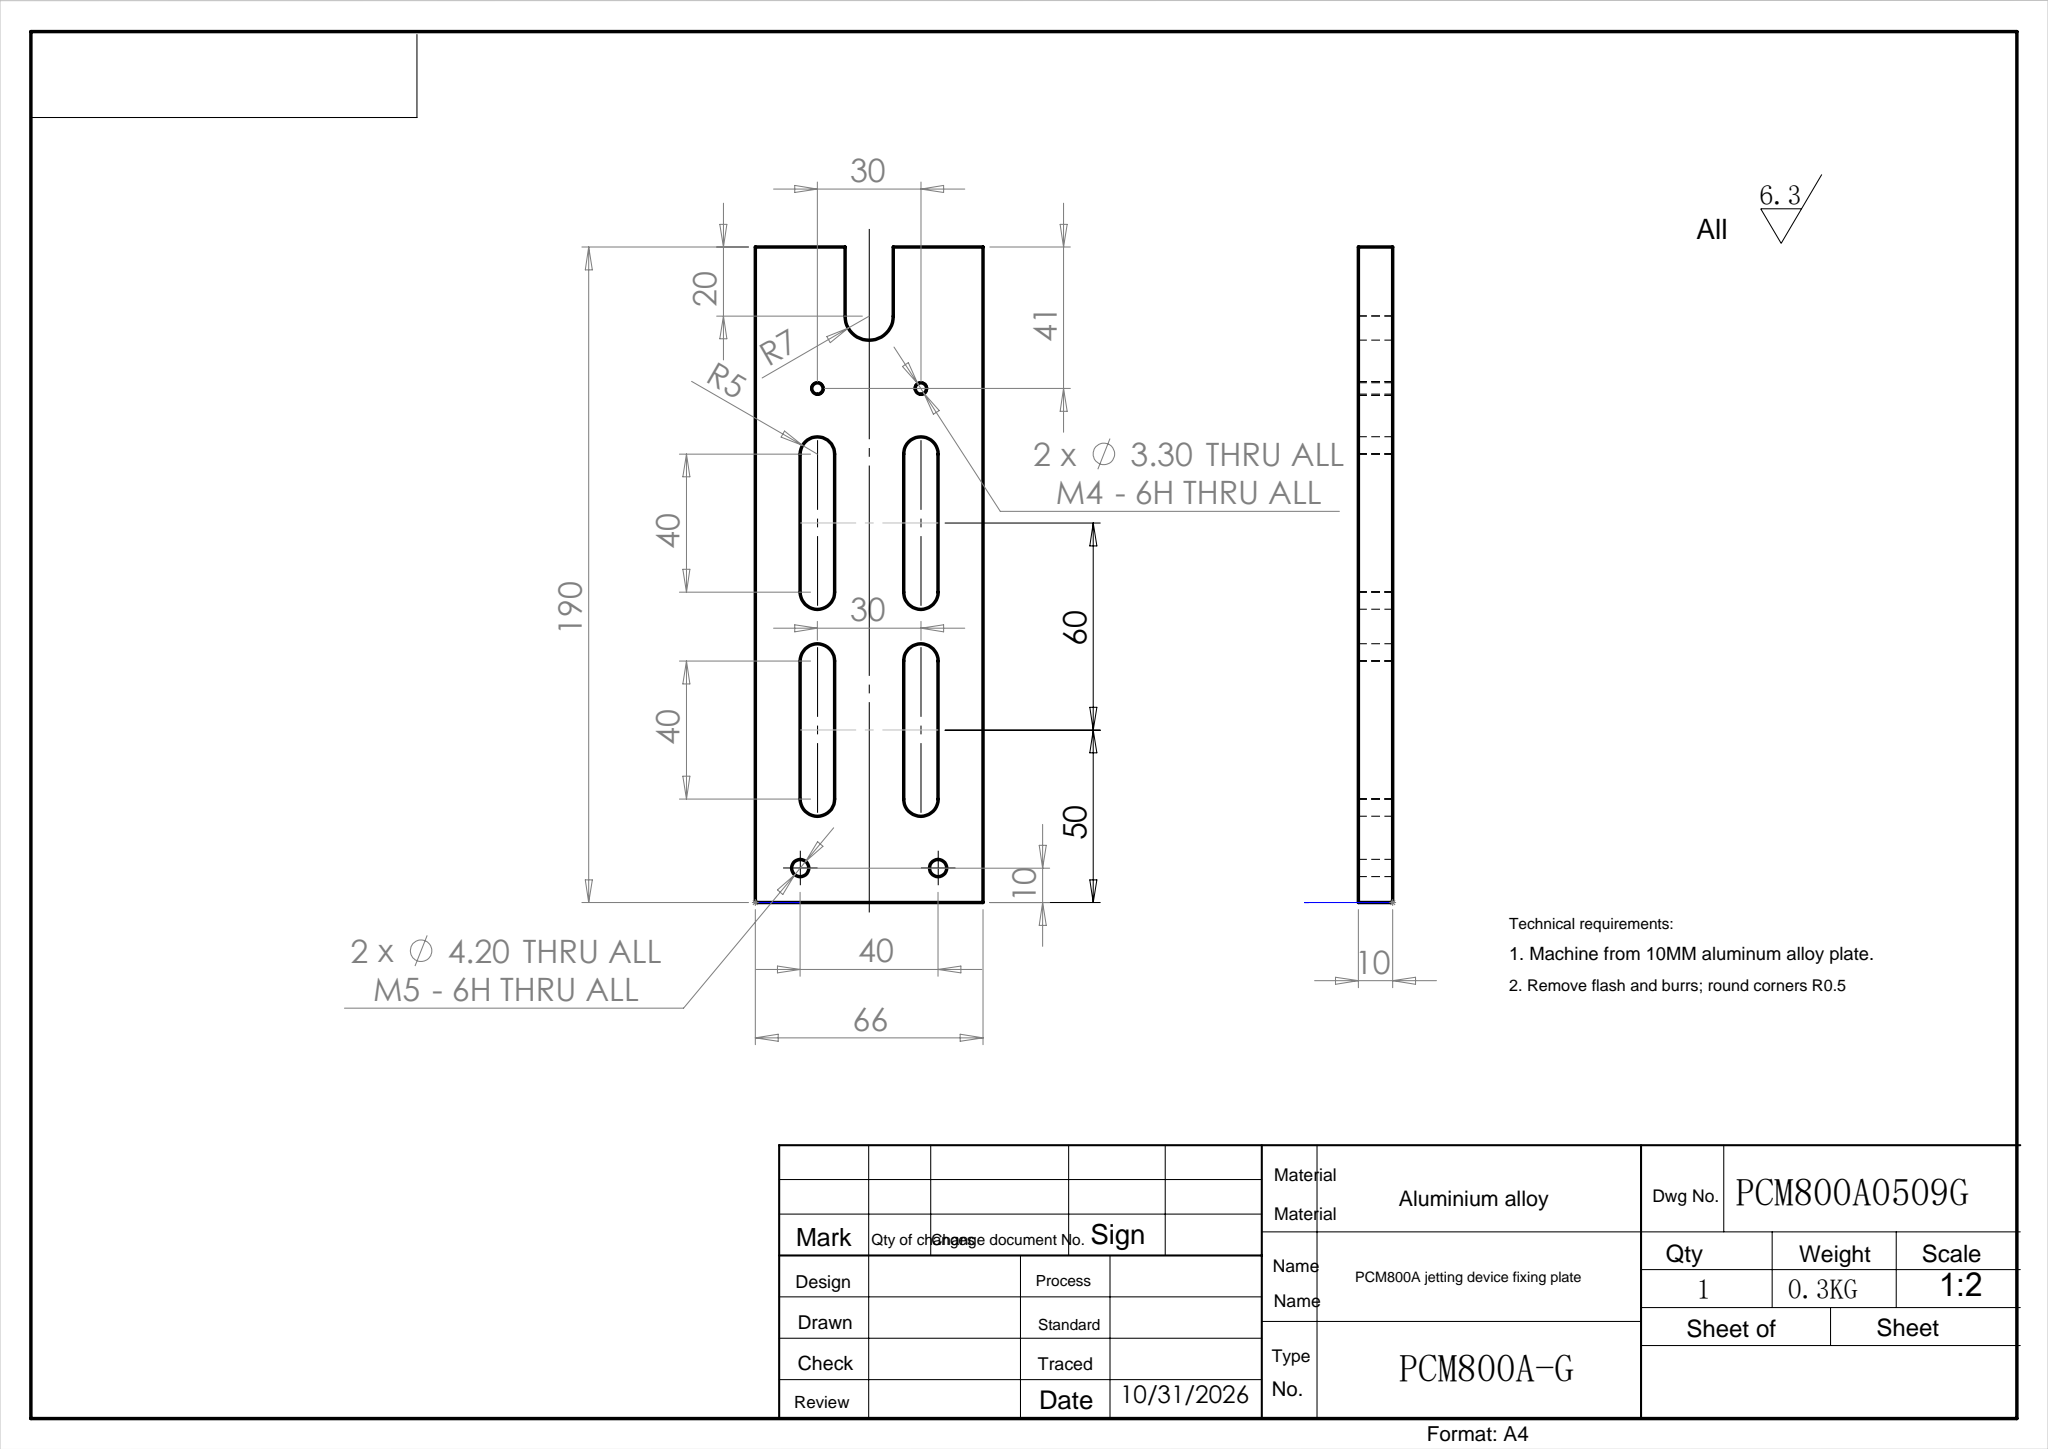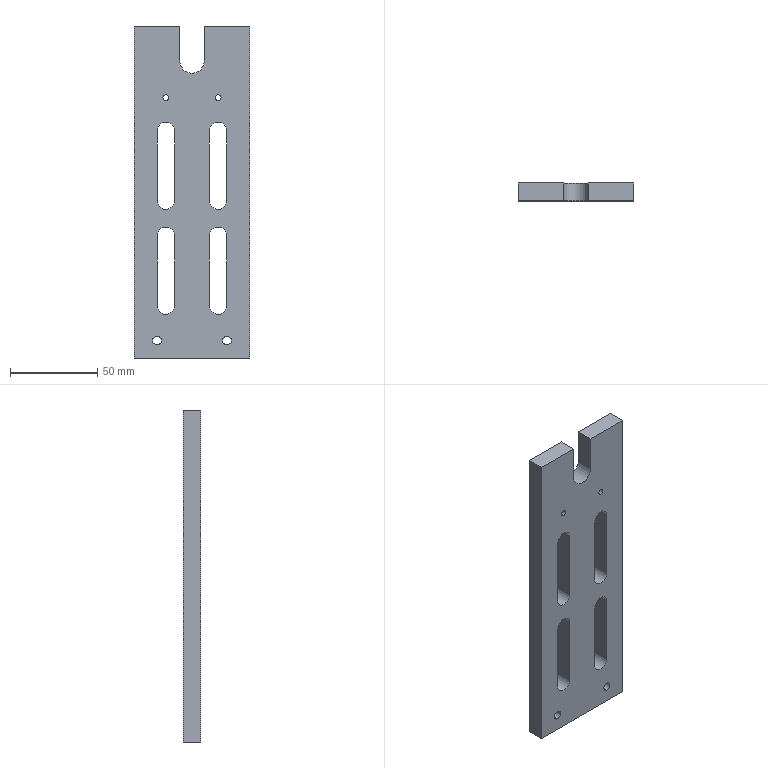Part | SolidWorks | features Cut 2, HoleWzd 2, Extrusion 1 | 1 solid | 34 faces | box 66 x 10 x 190 mm | volume 102125 mm3 | cylinder 17 | plane 17 | commonest cylinder face diameters 10 x8 3.3 x4 5 x4 14 x1